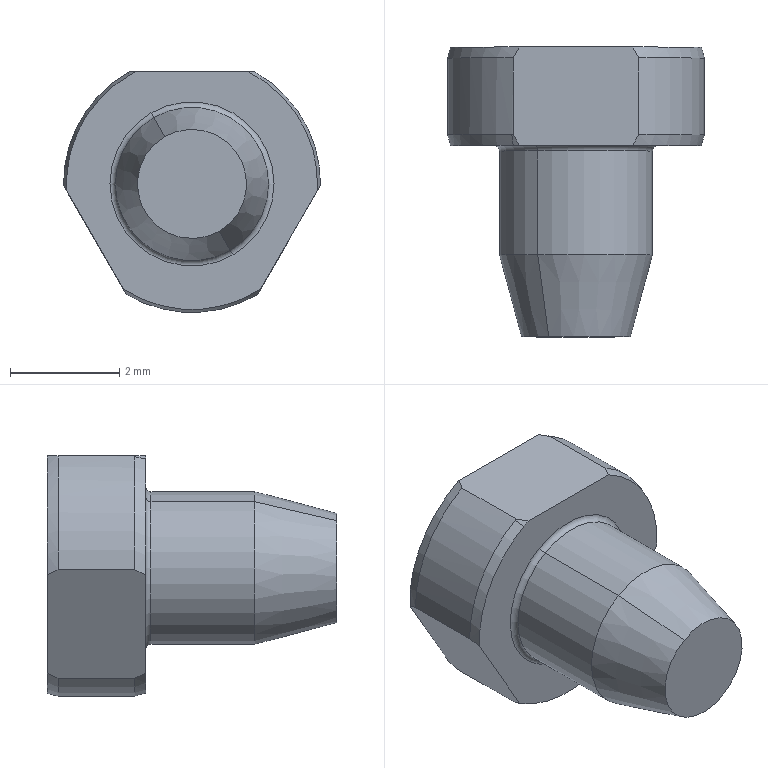Part | SolidWorks | features BaseBody 1 | 1 solid | 26 faces | box 4.7 x 5.3 x 4.4 mm | volume 46.239 mm3 | cone 10 | cylinder 6 | plane 6 | torus 2 | sphere 2 | commonest cylinder face diameters 4.7 x4 2.8 x2
STEP:
#1=CARTESIAN_POINT('',(229.999,165.3,-0.8644));
#2=VERTEX_POINT('',#1);
#3=CARTESIAN_POINT('',(229.001,165.3,0.8644));
#4=VERTEX_POINT('',#3);
#5=CARTESIAN_POINT('',(229.5,165.3,0.));
#6=DIRECTION('',(0.,-1.,0.));
#7=DIRECTION('',(0.5,0.,-0.866));
#8=AXIS2_PLACEMENT_3D('',#5,#6,#7);
#9=CIRCLE('',#8,0.9981);
#10=EDGE_CURVE('',#2,#4,#9,.T.);
#11=ORIENTED_EDGE('',*,*,#10,.F.);
#12=CARTESIAN_POINT('',(230.2,166.8,-1.212));
#13=VERTEX_POINT('',#12);
#14=CARTESIAN_POINT('',(229.999,165.3,-0.8644));
#15=DIRECTION('',(0.1294,0.9659,-0.2241));
#16=VECTOR('',#15,1000.);
#17=LINE('',#14,#16);
#18=EDGE_CURVE('',#2,#13,#17,.T.);
#19=ORIENTED_EDGE('',*,*,#18,.T.);
#20=CARTESIAN_POINT('',(228.8,166.8,1.212));
#21=VERTEX_POINT('',#20);
#22=CARTESIAN_POINT('',(229.5,166.8,0.));
#23=DIRECTION('',(0.,-1.,0.));
#24=DIRECTION('',(0.5,0.,-0.866));
#25=AXIS2_PLACEMENT_3D('',#22,#23,#24);
#26=CIRCLE('',#25,1.4);
#27=EDGE_CURVE('',#13,#21,#26,.T.);
#28=ORIENTED_EDGE('',*,*,#27,.T.);
#29=CARTESIAN_POINT('',(229.001,165.3,0.8644));
#30=DIRECTION('',(-0.1294,0.9659,0.2241));
#31=VECTOR('',#30,1000.);
#32=LINE('',#29,#31);
#33=EDGE_CURVE('',#4,#21,#32,.T.);
#34=ORIENTED_EDGE('',*,*,#33,.F.);
#35=EDGE_LOOP('',(#11,#19,#28,#34));
#36=FACE_OUTER_BOUND('',#35,.T.);
#37=CARTESIAN_POINT('',(229.5,165.3,0.));
#38=DIRECTION('',(0.,1.,0.));
#39=DIRECTION('',(-0.5,0.,0.866));
#40=AXIS2_PLACEMENT_3D('',#37,#38,#39);
#41=CONICAL_SURFACE('',#40,0.9981,0.2618);
#42=ADVANCED_FACE('',(#36),#41,.T.);
#43=CARTESIAN_POINT('',(230.2,168.7,-1.212));
#44=VERTEX_POINT('',#43);
#45=CARTESIAN_POINT('',(228.8,168.7,1.212));
#46=VERTEX_POINT('',#45);
#47=CARTESIAN_POINT('',(229.5,168.7,0.));
#48=DIRECTION('',(0.,-1.,0.));
#49=DIRECTION('',(0.5,0.,-0.866));
#50=AXIS2_PLACEMENT_3D('',#47,#48,#49);
#51=CIRCLE('',#50,1.4);
#52=EDGE_CURVE('',#44,#46,#51,.T.);
#53=ORIENTED_EDGE('',*,*,#52,.T.);
#54=CARTESIAN_POINT('',(228.8,164.118,1.212));
#55=DIRECTION('',(0.,-1.,0.));
#56=VECTOR('',#55,1000.);
#57=LINE('',#54,#56);
#58=EDGE_CURVE('',#46,#21,#57,.T.);
#59=ORIENTED_EDGE('',*,*,#58,.T.);
#60=ORIENTED_EDGE('',*,*,#27,.F.);
#61=CARTESIAN_POINT('',(230.2,164.118,-1.212));
#62=DIRECTION('',(0.,-1.,0.));
#63=VECTOR('',#62,1000.);
#64=LINE('',#61,#63);
#65=EDGE_CURVE('',#44,#13,#64,.T.);
#66=ORIENTED_EDGE('',*,*,#65,.F.);
#67=EDGE_LOOP('',(#53,#59,#60,#66));
#68=FACE_OUTER_BOUND('',#67,.T.);
#69=CARTESIAN_POINT('',(229.5,164.118,0.));
#70=DIRECTION('',(0.,-1.,0.));
#71=DIRECTION('',(0.5,0.,-0.866));
#72=AXIS2_PLACEMENT_3D('',#69,#70,#71);
#73=CYLINDRICAL_SURFACE('',#72,1.4);
#74=ADVANCED_FACE('',(#68),#73,.T.);
#75=CARTESIAN_POINT('',(229.5,168.7,0.));
#76=DIRECTION('',(0.,-1.,0.));
#77=DIRECTION('',(0.5,0.,-0.866));
#78=AXIS2_PLACEMENT_3D('',#75,#76,#77);
#79=CIRCLE('',#78,1.4);
#80=EDGE_CURVE('',#46,#44,#79,.T.);
#81=ORIENTED_EDGE('',*,*,#80,.F.);
#82=CARTESIAN_POINT('',(228.75,168.8,1.299));
#83=VERTEX_POINT('',#82);
#84=CARTESIAN_POINT('',(228.75,168.7,1.299));
#85=DIRECTION('',(0.866,0.,0.5));
#86=DIRECTION('',(0.5,0.,-0.866));
#87=AXIS2_PLACEMENT_3D('',#84,#85,#86);
#88=CIRCLE('',#87,0.1);
#89=EDGE_CURVE('',#46,#83,#88,.T.);
#90=ORIENTED_EDGE('',*,*,#89,.T.);
#91=CARTESIAN_POINT('',(230.25,168.8,-1.299));
#92=VERTEX_POINT('',#91);
#93=CARTESIAN_POINT('',(229.5,168.8,0.));
#94=DIRECTION('',(0.,-1.,0.));
#95=DIRECTION('',(0.5,0.,-0.866));
#96=AXIS2_PLACEMENT_3D('',#93,#94,#95);
#97=CIRCLE('',#96,1.5);
#98=EDGE_CURVE('',#83,#92,#97,.T.);
#99=ORIENTED_EDGE('',*,*,#98,.T.);
#100=CARTESIAN_POINT('',(230.25,168.7,-1.299));
#101=DIRECTION('',(-0.866,0.,-0.5));
#102=DIRECTION('',(-0.5,0.,0.866));
#103=AXIS2_PLACEMENT_3D('',#100,#101,#102);
#104=CIRCLE('',#103,0.1);
#105=EDGE_CURVE('',#44,#92,#104,.T.);
#106=ORIENTED_EDGE('',*,*,#105,.F.);
#107=EDGE_LOOP('',(#81,#90,#99,#106));
#108=FACE_OUTER_BOUND('',#107,.T.);
#109=CARTESIAN_POINT('',(229.5,168.7,0.));
#110=DIRECTION('',(0.,-1.,0.));
#111=DIRECTION('',(0.5,0.,-0.866));
#112=AXIS2_PLACEMENT_3D('',#109,#110,#111);
#113=TOROIDAL_SURFACE('',#112,1.5,0.1);
#114=ADVANCED_FACE('',(#108),#113,.F.);
#115=CARTESIAN_POINT('',(228.528,170.6,-0.5612));
#116=VERTEX_POINT('',#115);
#117=CARTESIAN_POINT('',(230.472,170.6,0.5612));
#118=VERTEX_POINT('',#117);
#119=CARTESIAN_POINT('',(229.5,170.6,0.));
#120=DIRECTION('',(0.,-1.,0.));
#121=DIRECTION('',(0.5,0.,-0.866));
#122=AXIS2_PLACEMENT_3D('',#119,#120,#121);
#123=CIRCLE('',#122,1.122);
#124=EDGE_CURVE('',#116,#118,#123,.T.);
#125=ORIENTED_EDGE('',*,*,#124,.F.);
#126=CARTESIAN_POINT('',(229.5,169.9,0.));
#127=VERTEX_POINT('',#126);
#128=CARTESIAN_POINT('',(229.5,171.15,0.));
#129=DIRECTION('',(-0.5,0.,0.866));
#130=DIRECTION('',(0.866,0.,0.5));
#131=AXIS2_PLACEMENT_3D('',#128,#129,#130);
#132=CIRCLE('',#131,1.25);
#133=EDGE_CURVE('',#116,#127,#132,.T.);
#134=ORIENTED_EDGE('',*,*,#133,.T.);
#135=CARTESIAN_POINT('',(229.5,171.15,0.));
#136=DIRECTION('',(0.5,0.,-0.866));
#137=DIRECTION('',(-0.866,0.,-0.5));
#138=AXIS2_PLACEMENT_3D('',#135,#136,#137);
#139=CIRCLE('',#138,1.25);
#140=EDGE_CURVE('',#118,#127,#139,.T.);
#141=ORIENTED_EDGE('',*,*,#140,.F.);
#142=EDGE_LOOP('',(#125,#134,#141));
#143=FACE_OUTER_BOUND('',#142,.T.);
#144=CARTESIAN_POINT('',(229.5,171.15,0.));
#145=DIRECTION('',(-0.5,0.,0.866));
#146=DIRECTION('',(0.866,0.,0.5));
#147=AXIS2_PLACEMENT_3D('',#144,#145,#146);
#148=SPHERICAL_SURFACE('',#147,1.25);
#149=ADVANCED_FACE('',(#143),#148,.F.);
#150=CARTESIAN_POINT('',(228.352,168.8,1.989));
#151=VERTEX_POINT('',#150);
#152=CARTESIAN_POINT('',(227.207,168.8,-0.1287));
#153=VERTEX_POINT('',#152);
#154=CARTESIAN_POINT('',(229.5,168.8,0.));
#155=DIRECTION('',(0.,-1.,0.));
#156=DIRECTION('',(0.5,0.,-0.866));
#157=AXIS2_PLACEMENT_3D('',#154,#155,#156);
#158=CIRCLE('',#157,2.296);
#159=EDGE_CURVE('',#151,#153,#158,.T.);
#160=ORIENTED_EDGE('',*,*,#159,.F.);
#161=CARTESIAN_POINT('',(228.325,169.,2.035));
#162=VERTEX_POINT('',#161);
#163=CARTESIAN_POINT('',(228.352,168.8,1.989));
#164=DIRECTION('',(-0.1294,0.9659,0.2241));
#165=VECTOR('',#164,1000.);
#166=LINE('',#163,#165);
#167=EDGE_CURVE('',#151,#162,#166,.T.);
#168=ORIENTED_EDGE('',*,*,#167,.T.);
#169=CARTESIAN_POINT('',(227.15,169.,-0.02996));
#170=VERTEX_POINT('',#169);
#171=CARTESIAN_POINT('',(229.5,169.,0.));
#172=DIRECTION('',(0.,-1.,0.));
#173=DIRECTION('',(0.5,0.,-0.866));
#174=AXIS2_PLACEMENT_3D('',#171,#172,#173);
#175=CIRCLE('',#174,2.35);
#176=EDGE_CURVE('',#162,#170,#175,.T.);
#177=ORIENTED_EDGE('',*,*,#176,.T.);
#178=CARTESIAN_POINT('',(227.15,169.,-0.02996));
#179=CARTESIAN_POINT('',(227.169,168.933,-0.0619));
#180=CARTESIAN_POINT('',(227.188,168.866,-0.09473));
#181=CARTESIAN_POINT('',(227.207,168.8,-0.1287));
#182=B_SPLINE_CURVE_WITH_KNOTS('',3,(#178,#179,#180,#181),.UNSPECIFIED.,.F.,.F.,(4,4),(0.001525,0.001756),.UNSPECIFIED.);
#183=EDGE_CURVE('',#170,#153,#182,.T.);
#184=ORIENTED_EDGE('',*,*,#183,.T.);
#185=EDGE_LOOP('',(#160,#168,#177,#184));
#186=FACE_OUTER_BOUND('',#185,.T.);
#187=CARTESIAN_POINT('',(229.5,168.8,0.));
#188=DIRECTION('',(0.,1.,0.));
#189=DIRECTION('',(-0.5,0.,0.866));
#190=AXIS2_PLACEMENT_3D('',#187,#188,#189);
#191=CONICAL_SURFACE('',#190,2.296,0.2618);
#192=ADVANCED_FACE('',(#186),#191,.T.);
#193=CARTESIAN_POINT('',(228.299,170.4,-2.02));
#194=VERTEX_POINT('',#193);
#195=CARTESIAN_POINT('',(230.675,170.4,-2.035));
#196=VERTEX_POINT('',#195);
#197=CARTESIAN_POINT('',(229.5,170.4,0.));
#198=DIRECTION('',(0.,-1.,0.));
#199=DIRECTION('',(0.5,0.,-0.866));
#200=AXIS2_PLACEMENT_3D('',#197,#198,#199);
#201=CIRCLE('',#200,2.35);
#202=EDGE_CURVE('',#194,#196,#201,.T.);
#203=ORIENTED_EDGE('',*,*,#202,.T.);
#204=CARTESIAN_POINT('',(230.675,169.,-2.035));
#205=VERTEX_POINT('',#204);
#206=CARTESIAN_POINT('',(230.675,164.118,-2.035));
#207=DIRECTION('',(0.,-1.,0.));
#208=VECTOR('',#207,1000.);
#209=LINE('',#206,#208);
#210=EDGE_CURVE('',#196,#205,#209,.T.);
#211=ORIENTED_EDGE('',*,*,#210,.T.);
#212=CARTESIAN_POINT('',(228.299,169.,-2.02));
#213=VERTEX_POINT('',#212);
#214=CARTESIAN_POINT('',(229.5,169.,0.));
#215=DIRECTION('',(0.,-1.,0.));
#216=DIRECTION('',(0.5,0.,-0.866));
#217=AXIS2_PLACEMENT_3D('',#214,#215,#216);
#218=CIRCLE('',#217,2.35);
#219=EDGE_CURVE('',#213,#205,#218,.T.);
#220=ORIENTED_EDGE('',*,*,#219,.F.);
#221=CARTESIAN_POINT('',(228.299,170.601,-2.02));
#222=DIRECTION('',(0.,-1.,0.));
#223=VECTOR('',#222,1000.);
#224=LINE('',#221,#223);
#225=EDGE_CURVE('',#194,#213,#224,.T.);
#226=ORIENTED_EDGE('',*,*,#225,.F.);
#227=EDGE_LOOP('',(#203,#211,#220,#226));
#228=FACE_OUTER_BOUND('',#227,.T.);
#229=CARTESIAN_POINT('',(229.5,164.118,0.));
#230=DIRECTION('',(0.,-1.,0.));
#231=DIRECTION('',(0.5,0.,-0.866));
#232=AXIS2_PLACEMENT_3D('',#229,#230,#231);
#233=CYLINDRICAL_SURFACE('',#232,2.35);
#234=ADVANCED_FACE('',(#228),#233,.T.);
#235=CARTESIAN_POINT('',(228.242,170.6,-1.921));
#236=VERTEX_POINT('',#235);
#237=CARTESIAN_POINT('',(230.648,170.6,-1.989));
#238=VERTEX_POINT('',#237);
#239=CARTESIAN_POINT('',(229.5,170.6,0.));
#240=DIRECTION('',(0.,-1.,0.));
#241=DIRECTION('',(0.5,0.,-0.866));
#242=AXIS2_PLACEMENT_3D('',#239,#240,#241);
#243=CIRCLE('',#242,2.296);
#244=EDGE_CURVE('',#236,#238,#243,.T.);
#245=ORIENTED_EDGE('',*,*,#244,.T.);
#246=CARTESIAN_POINT('',(230.675,170.4,-2.035));
#247=DIRECTION('',(0.1294,-0.9659,-0.2241));
#248=VECTOR('',#247,1000.);
#249=LINE('',#246,#248);
#250=EDGE_CURVE('',#238,#196,#249,.T.);
#251=ORIENTED_EDGE('',*,*,#250,.T.);
#252=ORIENTED_EDGE('',*,*,#202,.F.);
#253=CARTESIAN_POINT('',(228.299,170.4,-2.02));
#254=CARTESIAN_POINT('',(228.281,170.467,-1.988));
#255=CARTESIAN_POINT('',(228.262,170.534,-1.955));
#256=CARTESIAN_POINT('',(228.242,170.6,-1.921));
#257=B_SPLINE_CURVE_WITH_KNOTS('',3,(#253,#254,#255,#256),.UNSPECIFIED.,.F.,.F.,(4,4),(0.001525,0.001756),.UNSPECIFIED.);
#258=EDGE_CURVE('',#194,#236,#257,.T.);
#259=ORIENTED_EDGE('',*,*,#258,.T.);
#260=EDGE_LOOP('',(#245,#251,#252,#259));
#261=FACE_OUTER_BOUND('',#260,.T.);
#262=CARTESIAN_POINT('',(229.5,170.4,0.));
#263=DIRECTION('',(0.,-1.,0.));
#264=DIRECTION('',(0.5,0.,-0.866));
#265=AXIS2_PLACEMENT_3D('',#262,#263,#264);
#266=CONICAL_SURFACE('',#265,2.35,0.2618);
#267=ADVANCED_FACE('',(#261),#266,.T.);
#268=CARTESIAN_POINT('',(229.5,170.6,0.));
#269=DIRECTION('',(0.,-1.,0.));
#270=DIRECTION('',(0.5,0.,-0.866));
#271=AXIS2_PLACEMENT_3D('',#268,#269,#270);
#272=CIRCLE('',#271,1.122);
#273=EDGE_CURVE('',#118,#116,#272,.T.);
#274=ORIENTED_EDGE('',*,*,#273,.T.);
#275=ORIENTED_EDGE('',*,*,#124,.T.);
#276=EDGE_LOOP('',(#274,#275));
#277=FACE_BOUND('',#276,.T.);
#278=CARTESIAN_POINT('',(228.465,170.6,2.05));
#279=VERTEX_POINT('',#278);
#280=CARTESIAN_POINT('',(230.535,170.6,2.05));
#281=VERTEX_POINT('',#280);
#282=CARTESIAN_POINT('',(228.351,170.6,2.05));
#283=DIRECTION('',(1.,0.,-0.00002301));
#284=VECTOR('',#283,1000.);
#285=LINE('',#282,#284);
#286=EDGE_CURVE('',#279,#281,#285,.T.);
#287=ORIENTED_EDGE('',*,*,#286,.T.);
#288=CARTESIAN_POINT('',(231.793,170.6,-0.1288));
#289=VERTEX_POINT('',#288);
#290=CARTESIAN_POINT('',(229.5,170.6,0.));
#291=DIRECTION('',(0.,-1.,0.));
#292=DIRECTION('',(0.5,0.,-0.866));
#293=AXIS2_PLACEMENT_3D('',#290,#291,#292);
#294=CIRCLE('',#293,2.296);
#295=EDGE_CURVE('',#289,#281,#294,.T.);
#296=ORIENTED_EDGE('',*,*,#295,.F.);
#297=CARTESIAN_POINT('',(230.758,170.6,-1.921));
#298=VERTEX_POINT('',#297);
#299=CARTESIAN_POINT('',(231.85,170.6,-0.03007));
#300=DIRECTION('',(-0.5,0.,-0.866));
#301=VECTOR('',#300,1000.);
#302=LINE('',#299,#301);
#303=EDGE_CURVE('',#289,#298,#302,.T.);
#304=ORIENTED_EDGE('',*,*,#303,.T.);
#305=CARTESIAN_POINT('',(229.5,170.6,0.));
#306=DIRECTION('',(0.,-1.,0.));
#307=DIRECTION('',(0.5,0.,-0.866));
#308=AXIS2_PLACEMENT_3D('',#305,#306,#307);
#309=CIRCLE('',#308,2.296);
#310=EDGE_CURVE('',#238,#298,#309,.T.);
#311=ORIENTED_EDGE('',*,*,#310,.F.);
#312=ORIENTED_EDGE('',*,*,#244,.F.);
#313=CARTESIAN_POINT('',(227.207,170.6,-0.1287));
#314=VERTEX_POINT('',#313);
#315=CARTESIAN_POINT('',(228.299,170.6,-2.02));
#316=DIRECTION('',(-0.5,0.,0.866));
#317=VECTOR('',#316,1000.);
#318=LINE('',#315,#317);
#319=EDGE_CURVE('',#236,#314,#318,.T.);
#320=ORIENTED_EDGE('',*,*,#319,.T.);
#321=CARTESIAN_POINT('',(229.5,170.6,0.));
#322=DIRECTION('',(0.,-1.,0.));
#323=DIRECTION('',(0.5,0.,-0.866));
#324=AXIS2_PLACEMENT_3D('',#321,#322,#323);
#325=CIRCLE('',#324,2.296);
#326=EDGE_CURVE('',#279,#314,#325,.T.);
#327=ORIENTED_EDGE('',*,*,#326,.F.);
#328=EDGE_LOOP('',(#287,#296,#304,#311,#312,#320,#327));
#329=FACE_OUTER_BOUND('',#328,.T.);
#330=CARTESIAN_POINT('',(231.489,170.6,1.148));
#331=DIRECTION('',(0.,1.,0.));
#332=DIRECTION('',(-0.5,0.,0.866));
#333=AXIS2_PLACEMENT_3D('',#330,#331,#332);
#334=PLANE('',#333);
#335=ADVANCED_FACE('',(#277,#329),#334,.T.);
#336=CARTESIAN_POINT('',(230.649,170.4,2.05));
#337=VERTEX_POINT('',#336);
#338=CARTESIAN_POINT('',(230.535,170.6,2.05));
#339=CARTESIAN_POINT('',(230.574,170.534,2.05));
#340=CARTESIAN_POINT('',(230.612,170.467,2.05));
#341=CARTESIAN_POINT('',(230.649,170.4,2.05));
#342=B_SPLINE_CURVE_WITH_KNOTS('',3,(#338,#339,#340,#341),.UNSPECIFIED.,.F.,.F.,(4,4),(0.004642,0.004873),.UNSPECIFIED.);
#343=EDGE_CURVE('',#281,#337,#342,.T.);
#344=ORIENTED_EDGE('',*,*,#343,.T.);
#345=CARTESIAN_POINT('',(231.85,170.4,-0.03007));
#346=VERTEX_POINT('',#345);
#347=CARTESIAN_POINT('',(229.5,170.4,0.));
#348=DIRECTION('',(0.,-1.,0.));
#349=DIRECTION('',(0.5,0.,-0.866));
#350=AXIS2_PLACEMENT_3D('',#347,#348,#349);
#351=CIRCLE('',#350,2.35);
#352=EDGE_CURVE('',#346,#337,#351,.T.);
#353=ORIENTED_EDGE('',*,*,#352,.F.);
#354=CARTESIAN_POINT('',(231.85,170.4,-0.03007));
#355=CARTESIAN_POINT('',(231.831,170.467,-0.06201));
#356=CARTESIAN_POINT('',(231.812,170.534,-0.09484));
#357=CARTESIAN_POINT('',(231.793,170.6,-0.1288));
#358=B_SPLINE_CURVE_WITH_KNOTS('',3,(#354,#355,#356,#357),.UNSPECIFIED.,.F.,.F.,(4,4),(0.001525,0.001756),.UNSPECIFIED.);
#359=EDGE_CURVE('',#346,#289,#358,.T.);
#360=ORIENTED_EDGE('',*,*,#359,.T.);
#361=ORIENTED_EDGE('',*,*,#295,.T.);
#362=EDGE_LOOP('',(#344,#353,#360,#361));
#363=FACE_OUTER_BOUND('',#362,.T.);
#364=CARTESIAN_POINT('',(229.5,170.4,0.));
#365=DIRECTION('',(0.,-1.,0.));
#366=DIRECTION('',(0.5,0.,-0.866));
#367=AXIS2_PLACEMENT_3D('',#364,#365,#366);
#368=CONICAL_SURFACE('',#367,2.35,0.2618);
#369=ADVANCED_FACE('',(#363),#368,.T.);
#370=CARTESIAN_POINT('',(228.351,170.4,2.05));
#371=VERTEX_POINT('',#370);
#372=CARTESIAN_POINT('',(228.351,170.4,2.05));
#373=CARTESIAN_POINT('',(228.388,170.467,2.05));
#374=CARTESIAN_POINT('',(228.426,170.534,2.05));
#375=CARTESIAN_POINT('',(228.465,170.6,2.05));
#376=B_SPLINE_CURVE_WITH_KNOTS('',3,(#372,#373,#374,#375),.UNSPECIFIED.,.F.,.F.,(4,4),(0.001525,0.001756),.UNSPECIFIED.);
#377=EDGE_CURVE('',#371,#279,#376,.T.);
#378=ORIENTED_EDGE('',*,*,#377,.T.);
#379=ORIENTED_EDGE('',*,*,#326,.T.);
#380=CARTESIAN_POINT('',(227.15,170.4,-0.02996));
#381=VERTEX_POINT('',#380);
#382=CARTESIAN_POINT('',(227.207,170.6,-0.1287));
#383=CARTESIAN_POINT('',(227.188,170.534,-0.09476));
#384=CARTESIAN_POINT('',(227.169,170.467,-0.06188));
#385=CARTESIAN_POINT('',(227.15,170.4,-0.02996));
#386=B_SPLINE_CURVE_WITH_KNOTS('',3,(#382,#383,#384,#385),.UNSPECIFIED.,.F.,.F.,(4,4),(0.004642,0.004873),.UNSPECIFIED.);
#387=EDGE_CURVE('',#314,#381,#386,.T.);
#388=ORIENTED_EDGE('',*,*,#387,.T.);
#389=CARTESIAN_POINT('',(229.5,170.4,0.));
#390=DIRECTION('',(0.,-1.,0.));
#391=DIRECTION('',(0.5,0.,-0.866));
#392=AXIS2_PLACEMENT_3D('',#389,#390,#391);
#393=CIRCLE('',#392,2.35);
#394=EDGE_CURVE('',#371,#381,#393,.T.);
#395=ORIENTED_EDGE('',*,*,#394,.F.);
#396=EDGE_LOOP('',(#378,#379,#388,#395));
#397=FACE_OUTER_BOUND('',#396,.T.);
#398=CARTESIAN_POINT('',(229.5,170.4,0.));
#399=DIRECTION('',(0.,-1.,0.));
#400=DIRECTION('',(0.5,0.,-0.866));
#401=AXIS2_PLACEMENT_3D('',#398,#399,#400);
#402=CONICAL_SURFACE('',#401,2.35,0.2618);
#403=ADVANCED_FACE('',(#397),#402,.T.);
#404=ORIENTED_EDGE('',*,*,#250,.F.);
#405=ORIENTED_EDGE('',*,*,#310,.T.);
#406=CARTESIAN_POINT('',(230.701,170.4,-2.02));
#407=VERTEX_POINT('',#406);
#408=CARTESIAN_POINT('',(230.758,170.6,-1.921));
#409=CARTESIAN_POINT('',(230.738,170.534,-1.955));
#410=CARTESIAN_POINT('',(230.719,170.467,-1.988));
#411=CARTESIAN_POINT('',(230.701,170.4,-2.02));
#412=B_SPLINE_CURVE_WITH_KNOTS('',3,(#408,#409,#410,#411),.UNSPECIFIED.,.F.,.F.,(4,4),(0.004642,0.004873),.UNSPECIFIED.);
#413=EDGE_CURVE('',#298,#407,#412,.T.);
#414=ORIENTED_EDGE('',*,*,#413,.T.);
#415=CARTESIAN_POINT('',(229.5,170.4,0.));
#416=DIRECTION('',(0.,-1.,0.));
#417=DIRECTION('',(0.5,0.,-0.866));
#418=AXIS2_PLACEMENT_3D('',#415,#416,#417);
#419=CIRCLE('',#418,2.35);
#420=EDGE_CURVE('',#196,#407,#419,.T.);
#421=ORIENTED_EDGE('',*,*,#420,.F.);
#422=EDGE_LOOP('',(#404,#405,#414,#421));
#423=FACE_OUTER_BOUND('',#422,.T.);
#424=CARTESIAN_POINT('',(229.5,170.4,0.));
#425=DIRECTION('',(0.,-1.,0.));
#426=DIRECTION('',(0.5,0.,-0.866));
#427=AXIS2_PLACEMENT_3D('',#424,#425,#426);
#428=CONICAL_SURFACE('',#427,2.35,0.2618);
#429=ADVANCED_FACE('',(#423),#428,.T.);
#430=CARTESIAN_POINT('',(230.649,169.,2.05));
#431=VERTEX_POINT('',#430);
#432=CARTESIAN_POINT('',(230.649,170.601,2.05));
#433=DIRECTION('',(0.,-1.,0.));
#434=VECTOR('',#433,1000.);
#435=LINE('',#432,#434);
#436=EDGE_CURVE('',#337,#431,#435,.T.);
#437=ORIENTED_EDGE('',*,*,#436,.T.);
#438=CARTESIAN_POINT('',(231.85,169.,-0.03007));
#439=VERTEX_POINT('',#438);
#440=CARTESIAN_POINT('',(229.5,169.,0.));
#441=DIRECTION('',(0.,-1.,0.));
#442=DIRECTION('',(0.5,0.,-0.866));
#443=AXIS2_PLACEMENT_3D('',#440,#441,#442);
#444=CIRCLE('',#443,2.35);
#445=EDGE_CURVE('',#439,#431,#444,.T.);
#446=ORIENTED_EDGE('',*,*,#445,.F.);
#447=CARTESIAN_POINT('',(231.85,170.601,-0.03007));
#448=DIRECTION('',(0.,-1.,0.));
#449=VECTOR('',#448,1000.);
#450=LINE('',#447,#449);
#451=EDGE_CURVE('',#346,#439,#450,.T.);
#452=ORIENTED_EDGE('',*,*,#451,.F.);
#453=ORIENTED_EDGE('',*,*,#352,.T.);
#454=EDGE_LOOP('',(#437,#446,#452,#453));
#455=FACE_OUTER_BOUND('',#454,.T.);
#456=CARTESIAN_POINT('',(229.5,164.118,0.));
#457=DIRECTION('',(0.,-1.,0.));
#458=DIRECTION('',(0.5,0.,-0.866));
#459=AXIS2_PLACEMENT_3D('',#456,#457,#458);
#460=CYLINDRICAL_SURFACE('',#459,2.35);
#461=ADVANCED_FACE('',(#455),#460,.T.);
#462=CARTESIAN_POINT('',(228.351,169.,2.05));
#463=VERTEX_POINT('',#462);
#464=CARTESIAN_POINT('',(228.351,170.601,2.05));
#465=DIRECTION('',(0.,-1.,0.));
#466=VECTOR('',#465,1000.);
#467=LINE('',#464,#466);
#468=EDGE_CURVE('',#371,#463,#467,.T.);
#469=ORIENTED_EDGE('',*,*,#468,.F.);
#470=ORIENTED_EDGE('',*,*,#394,.T.);
#471=CARTESIAN_POINT('',(227.15,170.601,-0.02996));
#472=DIRECTION('',(0.,-1.,0.));
#473=VECTOR('',#472,1000.);
#474=LINE('',#471,#473);
#475=EDGE_CURVE('',#381,#170,#474,.T.);
#476=ORIENTED_EDGE('',*,*,#475,.T.);
#477=ORIENTED_EDGE('',*,*,#176,.F.);
#478=CARTESIAN_POINT('',(229.5,169.,0.));
#479=DIRECTION('',(0.,-1.,0.));
#480=DIRECTION('',(0.5,0.,-0.866));
#481=AXIS2_PLACEMENT_3D('',#478,#479,#480);
#482=CIRCLE('',#481,2.35);
#483=EDGE_CURVE('',#463,#162,#482,.T.);
#484=ORIENTED_EDGE('',*,*,#483,.F.);
#485=EDGE_LOOP('',(#469,#470,#476,#477,#484));
#486=FACE_OUTER_BOUND('',#485,.T.);
#487=CARTESIAN_POINT('',(229.5,164.118,0.));
#488=DIRECTION('',(0.,-1.,0.));
#489=DIRECTION('',(0.5,0.,-0.866));
#490=AXIS2_PLACEMENT_3D('',#487,#488,#489);
#491=CYLINDRICAL_SURFACE('',#490,2.35);
#492=ADVANCED_FACE('',(#486),#491,.T.);
#493=ORIENTED_EDGE('',*,*,#210,.F.);
#494=ORIENTED_EDGE('',*,*,#420,.T.);
#495=CARTESIAN_POINT('',(230.701,169.,-2.02));
#496=VERTEX_POINT('',#495);
#497=CARTESIAN_POINT('',(230.701,170.601,-2.02));
#498=DIRECTION('',(0.,-1.,0.));
#499=VECTOR('',#498,1000.);
#500=LINE('',#497,#499);
#501=EDGE_CURVE('',#407,#496,#500,.T.);
#502=ORIENTED_EDGE('',*,*,#501,.T.);
#503=CARTESIAN_POINT('',(229.5,169.,0.));
#504=DIRECTION('',(0.,-1.,0.));
#505=DIRECTION('',(0.5,0.,-0.866));
#506=AXIS2_PLACEMENT_3D('',#503,#504,#505);
#507=CIRCLE('',#506,2.35);
#508=EDGE_CURVE('',#205,#496,#507,.T.);
#509=ORIENTED_EDGE('',*,*,#508,.F.);
#510=EDGE_LOOP('',(#493,#494,#502,#509));
#511=FACE_OUTER_BOUND('',#510,.T.);
#512=CARTESIAN_POINT('',(229.5,164.118,0.));
#513=DIRECTION('',(0.,-1.,0.));
#514=DIRECTION('',(0.5,0.,-0.866));
#515=AXIS2_PLACEMENT_3D('',#512,#513,#514);
#516=CYLINDRICAL_SURFACE('',#515,2.35);
#517=ADVANCED_FACE('',(#511),#516,.T.);
#518=ORIENTED_EDGE('',*,*,#167,.F.);
#519=CARTESIAN_POINT('',(228.465,168.8,2.05));
#520=VERTEX_POINT('',#519);
#521=CARTESIAN_POINT('',(229.5,168.8,0.));
#522=DIRECTION('',(0.,-1.,0.));
#523=DIRECTION('',(0.5,0.,-0.866));
#524=AXIS2_PLACEMENT_3D('',#521,#522,#523);
#525=CIRCLE('',#524,2.296);
#526=EDGE_CURVE('',#520,#151,#525,.T.);
#527=ORIENTED_EDGE('',*,*,#526,.F.);
#528=CARTESIAN_POINT('',(228.465,168.8,2.05));
#529=CARTESIAN_POINT('',(228.426,168.866,2.05));
#530=CARTESIAN_POINT('',(228.388,168.933,2.05));
#531=CARTESIAN_POINT('',(228.351,169.,2.05));
#532=B_SPLINE_CURVE_WITH_KNOTS('',3,(#528,#529,#530,#531),.UNSPECIFIED.,.F.,.F.,(4,4),(0.004642,0.004873),.UNSPECIFIED.);
#533=EDGE_CURVE('',#520,#463,#532,.T.);
#534=ORIENTED_EDGE('',*,*,#533,.T.);
#535=ORIENTED_EDGE('',*,*,#483,.T.);
#536=EDGE_LOOP('',(#518,#527,#534,#535));
#537=FACE_OUTER_BOUND('',#536,.T.);
#538=CARTESIAN_POINT('',(229.5,168.8,0.));
#539=DIRECTION('',(0.,1.,0.));
#540=DIRECTION('',(-0.5,0.,0.866));
#541=AXIS2_PLACEMENT_3D('',#538,#539,#540);
#542=CONICAL_SURFACE('',#541,2.296,0.2618);
#543=ADVANCED_FACE('',(#537),#542,.T.);
#544=CARTESIAN_POINT('',(230.535,168.8,2.05));
#545=VERTEX_POINT('',#544);
#546=CARTESIAN_POINT('',(230.649,169.,2.05));
#547=CARTESIAN_POINT('',(230.612,168.933,2.05));
#548=CARTESIAN_POINT('',(230.574,168.866,2.05));
#549=CARTESIAN_POINT('',(230.535,168.8,2.05));
#550=B_SPLINE_CURVE_WITH_KNOTS('',3,(#546,#547,#548,#549),.UNSPECIFIED.,.F.,.F.,(4,4),(0.001525,0.001756),.UNSPECIFIED.);
#551=EDGE_CURVE('',#431,#545,#550,.T.);
#552=ORIENTED_EDGE('',*,*,#551,.T.);
#553=CARTESIAN_POINT('',(231.793,168.8,-0.1288));
#554=VERTEX_POINT('',#553);
#555=CARTESIAN_POINT('',(229.5,168.8,0.));
#556=DIRECTION('',(0.,-1.,0.));
#557=DIRECTION('',(0.5,0.,-0.866));
#558=AXIS2_PLACEMENT_3D('',#555,#556,#557);
#559=CIRCLE('',#558,2.296);
#560=EDGE_CURVE('',#554,#545,#559,.T.);
#561=ORIENTED_EDGE('',*,*,#560,.F.);
#562=CARTESIAN_POINT('',(231.793,168.8,-0.1288));
#563=CARTESIAN_POINT('',(231.812,168.866,-0.09486));
#564=CARTESIAN_POINT('',(231.831,168.933,-0.06198));
#565=CARTESIAN_POINT('',(231.85,169.,-0.03007));
#566=B_SPLINE_CURVE_WITH_KNOTS('',3,(#562,#563,#564,#565),.UNSPECIFIED.,.F.,.F.,(4,4),(0.004642,0.004873),.UNSPECIFIED.);
#567=EDGE_CURVE('',#554,#439,#566,.T.);
#568=ORIENTED_EDGE('',*,*,#567,.T.);
#569=ORIENTED_EDGE('',*,*,#445,.T.);
#570=EDGE_LOOP('',(#552,#561,#568,#569));
#571=FACE_OUTER_BOUND('',#570,.T.);
#572=CARTESIAN_POINT('',(229.5,168.8,0.));
#573=DIRECTION('',(0.,1.,0.));
#574=DIRECTION('',(-0.5,0.,0.866));
#575=AXIS2_PLACEMENT_3D('',#572,#573,#574);
#576=CONICAL_SURFACE('',#575,2.296,0.2618);
#577=ADVANCED_FACE('',(#571),#576,.T.);
#578=CARTESIAN_POINT('',(230.758,168.8,-1.921));
#579=VERTEX_POINT('',#578);
#580=CARTESIAN_POINT('',(230.701,169.,-2.02));
#581=CARTESIAN_POINT('',(230.719,168.933,-1.988));
#582=CARTESIAN_POINT('',(230.738,168.866,-1.955));
#583=CARTESIAN_POINT('',(230.758,168.8,-1.921));
#584=B_SPLINE_CURVE_WITH_KNOTS('',3,(#580,#581,#582,#583),.UNSPECIFIED.,.F.,.F.,(4,4),(0.001525,0.001756),.UNSPECIFIED.);
#585=EDGE_CURVE('',#496,#579,#584,.T.);
#586=ORIENTED_EDGE('',*,*,#585,.T.);
#587=CARTESIAN_POINT('',(228.242,168.8,-1.921));
#588=VERTEX_POINT('',#587);
#589=CARTESIAN_POINT('',(229.5,168.8,0.));
#590=DIRECTION('',(0.,-1.,0.));
#591=DIRECTION('',(0.5,0.,-0.866));
#592=AXIS2_PLACEMENT_3D('',#589,#590,#591);
#593=CIRCLE('',#592,2.296);
#594=EDGE_CURVE('',#588,#579,#593,.T.);
#595=ORIENTED_EDGE('',*,*,#594,.F.);
#596=CARTESIAN_POINT('',(228.242,168.8,-1.921));
#597=CARTESIAN_POINT('',(228.262,168.866,-1.955));
#598=CARTESIAN_POINT('',(228.281,168.933,-1.988));
#599=CARTESIAN_POINT('',(228.299,169.,-2.02));
#600=B_SPLINE_CURVE_WITH_KNOTS('',3,(#596,#597,#598,#599),.UNSPECIFIED.,.F.,.F.,(4,4),(0.004642,0.004873),.UNSPECIFIED.);
#601=EDGE_CURVE('',#588,#213,#600,.T.);
#602=ORIENTED_EDGE('',*,*,#601,.T.);
#603=ORIENTED_EDGE('',*,*,#219,.T.);
#604=ORIENTED_EDGE('',*,*,#508,.T.);
#605=EDGE_LOOP('',(#586,#595,#602,#603,#604));
#606=FACE_OUTER_BOUND('',#605,.T.);
#607=CARTESIAN_POINT('',(229.5,168.8,0.));
#608=DIRECTION('',(0.,1.,0.));
#609=DIRECTION('',(-0.5,0.,0.866));
#610=AXIS2_PLACEMENT_3D('',#607,#608,#609);
#611=CONICAL_SURFACE('',#610,2.296,0.2618);
#612=ADVANCED_FACE('',(#606),#611,.T.);
#613=CARTESIAN_POINT('',(229.5,168.8,0.));
#614=DIRECTION('',(0.,-1.,0.));
#615=DIRECTION('',(0.5,0.,-0.866));
#616=AXIS2_PLACEMENT_3D('',#613,#614,#615);
#617=CIRCLE('',#616,1.5);
#618=EDGE_CURVE('',#92,#83,#617,.T.);
#619=ORIENTED_EDGE('',*,*,#618,.F.);
#620=ORIENTED_EDGE('',*,*,#98,.F.);
#621=EDGE_LOOP('',(#619,#620));
#622=FACE_BOUND('',#621,.T.);
#623=CARTESIAN_POINT('',(228.351,168.8,2.05));
#624=DIRECTION('',(-1.,0.,0.00002301));
#625=VECTOR('',#624,1000.);
#626=LINE('',#623,#625);
#627=EDGE_CURVE('',#545,#520,#626,.T.);
#628=ORIENTED_EDGE('',*,*,#627,.T.);
#629=ORIENTED_EDGE('',*,*,#526,.T.);
#630=ORIENTED_EDGE('',*,*,#159,.T.);
#631=CARTESIAN_POINT('',(228.299,168.8,-2.02));
#632=DIRECTION('',(0.5,0.,-0.866));
#633=VECTOR('',#632,1000.);
#634=LINE('',#631,#633);
#635=EDGE_CURVE('',#153,#588,#634,.T.);
#636=ORIENTED_EDGE('',*,*,#635,.T.);
#637=ORIENTED_EDGE('',*,*,#594,.T.);
#638=CARTESIAN_POINT('',(231.85,168.8,-0.03007));
#639=DIRECTION('',(0.5,0.,0.866));
#640=VECTOR('',#639,1000.);
#641=LINE('',#638,#640);
#642=EDGE_CURVE('',#579,#554,#641,.T.);
#643=ORIENTED_EDGE('',*,*,#642,.T.);
#644=ORIENTED_EDGE('',*,*,#560,.T.);
#645=EDGE_LOOP('',(#628,#629,#630,#636,#637,#643,#644));
#646=FACE_OUTER_BOUND('',#645,.T.);
#647=CARTESIAN_POINT('',(230.799,168.8,0.75));
#648=DIRECTION('',(0.,-1.,0.));
#649=DIRECTION('',(0.5,0.,-0.866));
#650=AXIS2_PLACEMENT_3D('',#647,#648,#649);
#651=PLANE('',#650);
#652=ADVANCED_FACE('',(#622,#646),#651,.T.);
#653=ORIENTED_EDGE('',*,*,#133,.F.);
#654=ORIENTED_EDGE('',*,*,#273,.F.);
#655=ORIENTED_EDGE('',*,*,#140,.T.);
#656=EDGE_LOOP('',(#653,#654,#655));
#657=FACE_OUTER_BOUND('',#656,.T.);
#658=CARTESIAN_POINT('',(229.5,171.15,0.));
#659=DIRECTION('',(-0.5,0.,0.866));
#660=DIRECTION('',(0.866,0.,0.5));
#661=AXIS2_PLACEMENT_3D('',#658,#659,#660);
#662=SPHERICAL_SURFACE('',#661,1.25);
#663=ADVANCED_FACE('',(#657),#662,.F.);
#664=ORIENTED_EDGE('',*,*,#89,.F.);
#665=ORIENTED_EDGE('',*,*,#52,.F.);
#666=ORIENTED_EDGE('',*,*,#105,.T.);
#667=ORIENTED_EDGE('',*,*,#618,.T.);
#668=EDGE_LOOP('',(#664,#665,#666,#667));
#669=FACE_OUTER_BOUND('',#668,.T.);
#670=CARTESIAN_POINT('',(229.5,168.7,0.));
#671=DIRECTION('',(0.,-1.,0.));
#672=DIRECTION('',(0.5,0.,-0.866));
#673=AXIS2_PLACEMENT_3D('',#670,#671,#672);
#674=TOROIDAL_SURFACE('',#673,1.5,0.1);
#675=ADVANCED_FACE('',(#669),#674,.F.);
#676=ORIENTED_EDGE('',*,*,#58,.F.);
#677=ORIENTED_EDGE('',*,*,#80,.T.);
#678=ORIENTED_EDGE('',*,*,#65,.T.);
#679=CARTESIAN_POINT('',(229.5,166.8,0.));
#680=DIRECTION('',(0.,-1.,0.));
#681=DIRECTION('',(0.5,0.,-0.866));
#682=AXIS2_PLACEMENT_3D('',#679,#680,#681);
#683=CIRCLE('',#682,1.4);
#684=EDGE_CURVE('',#21,#13,#683,.T.);
#685=ORIENTED_EDGE('',*,*,#684,.F.);
#686=EDGE_LOOP('',(#676,#677,#678,#685));
#687=FACE_OUTER_BOUND('',#686,.T.);
#688=CARTESIAN_POINT('',(229.5,164.118,0.));
#689=DIRECTION('',(0.,-1.,0.));
#690=DIRECTION('',(0.5,0.,-0.866));
#691=AXIS2_PLACEMENT_3D('',#688,#689,#690);
#692=CYLINDRICAL_SURFACE('',#691,1.4);
#693=ADVANCED_FACE('',(#687),#692,.T.);
#694=ORIENTED_EDGE('',*,*,#18,.F.);
#695=CARTESIAN_POINT('',(229.5,165.3,0.));
#696=DIRECTION('',(0.,-1.,0.));
#697=DIRECTION('',(0.5,0.,-0.866));
#698=AXIS2_PLACEMENT_3D('',#695,#696,#697);
#699=CIRCLE('',#698,0.9981);
#700=EDGE_CURVE('',#4,#2,#699,.T.);
#701=ORIENTED_EDGE('',*,*,#700,.F.);
#702=ORIENTED_EDGE('',*,*,#33,.T.);
#703=ORIENTED_EDGE('',*,*,#684,.T.);
#704=EDGE_LOOP('',(#694,#701,#702,#703));
#705=FACE_OUTER_BOUND('',#704,.T.);
#706=CARTESIAN_POINT('',(229.5,165.3,0.));
#707=DIRECTION('',(0.,1.,0.));
#708=DIRECTION('',(-0.5,0.,0.866));
#709=AXIS2_PLACEMENT_3D('',#706,#707,#708);
#710=CONICAL_SURFACE('',#709,0.9981,0.2618);
#711=ADVANCED_FACE('',(#705),#710,.T.);
#712=ORIENTED_EDGE('',*,*,#700,.T.);
#713=ORIENTED_EDGE('',*,*,#10,.T.);
#714=EDGE_LOOP('',(#712,#713));
#715=FACE_OUTER_BOUND('',#714,.T.);
#716=CARTESIAN_POINT('',(229.5,165.3,0.));
#717=DIRECTION('',(0.,-1.,0.));
#718=DIRECTION('',(0.5,0.,-0.866));
#719=AXIS2_PLACEMENT_3D('',#716,#717,#718);
#720=PLANE('',#719);
#721=ADVANCED_FACE('',(#715),#720,.T.);
#722=ORIENTED_EDGE('',*,*,#258,.F.);
#723=ORIENTED_EDGE('',*,*,#225,.T.);
#724=ORIENTED_EDGE('',*,*,#601,.F.);
#725=ORIENTED_EDGE('',*,*,#635,.F.);
#726=ORIENTED_EDGE('',*,*,#183,.F.);
#727=ORIENTED_EDGE('',*,*,#475,.F.);
#728=ORIENTED_EDGE('',*,*,#387,.F.);
#729=ORIENTED_EDGE('',*,*,#319,.F.);
#730=EDGE_LOOP('',(#722,#723,#724,#725,#726,#727,#728,#729));
#731=FACE_OUTER_BOUND('',#730,.T.);
#732=CARTESIAN_POINT('',(228.299,170.601,-2.02));
#733=DIRECTION('',(0.866,0.,0.5));
#734=DIRECTION('',(0.5,0.,-0.866));
#735=AXIS2_PLACEMENT_3D('',#732,#733,#734);
#736=PLANE('',#735);
#737=ADVANCED_FACE('',(#731),#736,.F.);
#738=ORIENTED_EDGE('',*,*,#359,.F.);
#739=ORIENTED_EDGE('',*,*,#451,.T.);
#740=ORIENTED_EDGE('',*,*,#567,.F.);
#741=ORIENTED_EDGE('',*,*,#642,.F.);
#742=ORIENTED_EDGE('',*,*,#585,.F.);
#743=ORIENTED_EDGE('',*,*,#501,.F.);
#744=ORIENTED_EDGE('',*,*,#413,.F.);
#745=ORIENTED_EDGE('',*,*,#303,.F.);
#746=EDGE_LOOP('',(#738,#739,#740,#741,#742,#743,#744,#745));
#747=FACE_OUTER_BOUND('',#746,.T.);
#748=CARTESIAN_POINT('',(231.85,170.601,-0.03007));
#749=DIRECTION('',(-0.866,0.,0.5));
#750=DIRECTION('',(0.5,0.,0.866));
#751=AXIS2_PLACEMENT_3D('',#748,#749,#750);
#752=PLANE('',#751);
#753=ADVANCED_FACE('',(#747),#752,.F.);
#754=ORIENTED_EDGE('',*,*,#377,.F.);
#755=ORIENTED_EDGE('',*,*,#468,.T.);
#756=ORIENTED_EDGE('',*,*,#533,.F.);
#757=ORIENTED_EDGE('',*,*,#627,.F.);
#758=ORIENTED_EDGE('',*,*,#551,.F.);
#759=ORIENTED_EDGE('',*,*,#436,.F.);
#760=ORIENTED_EDGE('',*,*,#343,.F.);
#761=ORIENTED_EDGE('',*,*,#286,.F.);
#762=EDGE_LOOP('',(#754,#755,#756,#757,#758,#759,#760,#761));
#763=FACE_OUTER_BOUND('',#762,.T.);
#764=CARTESIAN_POINT('',(228.351,170.601,2.05));
#765=DIRECTION('',(-0.00002301,0.,-1.));
#766=DIRECTION('',(-1.,0.,0.00002301));
#767=AXIS2_PLACEMENT_3D('',#764,#765,#766);
#768=PLANE('',#767);
#769=ADVANCED_FACE('',(#763),#768,.F.);
#770=CLOSED_SHELL('',(#42,#74,#114,#149,#192,#234,#267,#335,#369,#403,#429,#461,#492,#517,#543,#577,#612,#652,#663,#675,#693,#711,#721,#737,#753,#769));
#771=MANIFOLD_SOLID_BREP('',#770);
#772=CARTESIAN_POINT('',(0.,0.,0.));
#773=DIRECTION('',(0.,0.,1.));
#774=DIRECTION('',(1.,0.,0.));
#775=AXIS2_PLACEMENT_3D('',#772,#773,#774);
#776=(LENGTH_UNIT()NAMED_UNIT(*)SI_UNIT(.MILLI.,.METRE.));
#777=UNCERTAINTY_MEASURE_WITH_UNIT(LENGTH_MEASURE(0.00001),#776,'','');
#778=(NAMED_UNIT(*)PLANE_ANGLE_UNIT()SI_UNIT($,.RADIAN.));
#779=(NAMED_UNIT(*)SI_UNIT($,.STERADIAN.)SOLID_ANGLE_UNIT());
#780=(GEOMETRIC_REPRESENTATION_CONTEXT(3)GLOBAL_UNCERTAINTY_ASSIGNED_CONTEXT((#777))GLOBAL_UNIT_ASSIGNED_CONTEXT((#776,#778,#779))REPRESENTATION_CONTEXT('',''));
#781=ADVANCED_BREP_SHAPE_REPRESENTATION('',(#771,#775),#780);